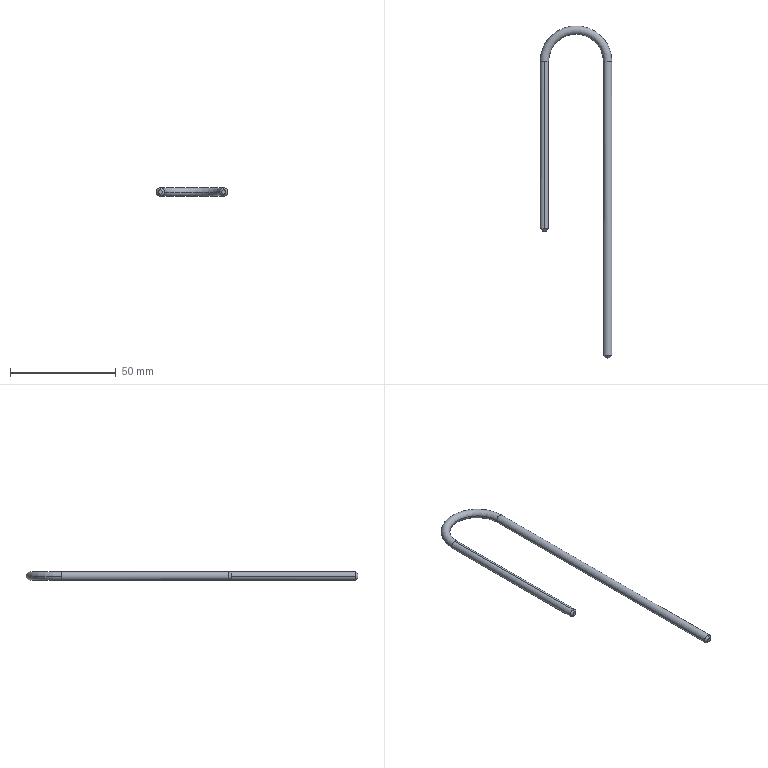Part | STEP file | MT-COMBO-119-S045 | 1 solid | 12 faces | box 34 x 157 x 4 mm | volume 3346 mm3 | cone 4 | cylinder 4 | torus 2 | plane 2 | commonest cylinder face diameters 4 x4
STEP:
#1=CARTESIAN_POINT('',(0.,80.,-2.));
#2=VERTEX_POINT('',#1);
#3=CARTESIAN_POINT('',(-2.,80.,0.));
#4=VERTEX_POINT('',#3);
#5=CARTESIAN_POINT('',(0.,80.,0.));
#6=DIRECTION('',(0.,1.,0.));
#7=DIRECTION('',(0.,0.,1.));
#8=AXIS2_PLACEMENT_3D('',#5,#6,#7);
#9=CIRCLE('',#8,2.);
#10=EDGE_CURVE('',#2,#4,#9,.T.);
#11=ORIENTED_EDGE('',*,*,#10,.T.);
#12=CARTESIAN_POINT('',(32.,80.,0.));
#13=VERTEX_POINT('',#12);
#14=CARTESIAN_POINT('',(15.,80.,0.));
#15=DIRECTION('',(0.,0.,-1.));
#16=DIRECTION('',(-1.,0.,0.));
#17=AXIS2_PLACEMENT_3D('',#14,#15,#16);
#18=CIRCLE('',#17,17.);
#19=EDGE_CURVE('',#4,#13,#18,.T.);
#20=ORIENTED_EDGE('',*,*,#19,.T.);
#21=CARTESIAN_POINT('',(28.,80.,0.));
#22=VERTEX_POINT('',#21);
#23=CARTESIAN_POINT('',(30.,80.,0.));
#24=DIRECTION('',(0.,-1.,0.));
#25=DIRECTION('',(0.,0.,1.));
#26=AXIS2_PLACEMENT_3D('',#23,#24,#25);
#27=CIRCLE('',#26,2.);
#28=EDGE_CURVE('',#22,#13,#27,.T.);
#29=ORIENTED_EDGE('',*,*,#28,.F.);
#30=CARTESIAN_POINT('',(2.,80.,0.));
#31=VERTEX_POINT('',#30);
#32=CARTESIAN_POINT('',(15.,80.,0.));
#33=DIRECTION('',(0.,0.,-1.));
#34=DIRECTION('',(-1.,0.,0.));
#35=AXIS2_PLACEMENT_3D('',#32,#33,#34);
#36=CIRCLE('',#35,13.);
#37=EDGE_CURVE('',#31,#22,#36,.T.);
#38=ORIENTED_EDGE('',*,*,#37,.F.);
#39=CARTESIAN_POINT('',(0.,80.,0.));
#40=DIRECTION('',(0.,1.,0.));
#41=DIRECTION('',(0.,0.,1.));
#42=AXIS2_PLACEMENT_3D('',#39,#40,#41);
#43=CIRCLE('',#42,2.);
#44=EDGE_CURVE('',#31,#2,#43,.T.);
#45=ORIENTED_EDGE('',*,*,#44,.T.);
#46=EDGE_LOOP('',(#11,#20,#29,#38,#45));
#47=FACE_OUTER_BOUND('',#46,.T.);
#48=CARTESIAN_POINT('',(15.,80.,0.));
#49=DIRECTION('',(0.,0.,-1.));
#50=DIRECTION('',(-1.,0.,0.));
#51=AXIS2_PLACEMENT_3D('',#48,#49,#50);
#52=TOROIDAL_SURFACE('',#51,15.,2.);
#53=ADVANCED_FACE('',(#47),#52,.T.);
#54=CARTESIAN_POINT('',(0.,0.,-1.));
#55=VERTEX_POINT('',#54);
#56=CARTESIAN_POINT('',(0.,0.,1.));
#57=VERTEX_POINT('',#56);
#58=CARTESIAN_POINT('',(0.,0.,0.));
#59=DIRECTION('',(0.,-1.,0.));
#60=DIRECTION('',(0.,0.,1.));
#61=AXIS2_PLACEMENT_3D('',#58,#59,#60);
#62=CIRCLE('',#61,1.);
#63=EDGE_CURVE('',#55,#57,#62,.T.);
#64=ORIENTED_EDGE('',*,*,#63,.F.);
#65=CARTESIAN_POINT('',(0.,1.,-2.));
#66=VERTEX_POINT('',#65);
#67=CARTESIAN_POINT('',(0.,1.,-2.));
#68=DIRECTION('',(0.,0.7071,-0.7071));
#69=VECTOR('',#68,1000.);
#70=LINE('',#67,#69);
#71=EDGE_CURVE('',#55,#66,#70,.T.);
#72=ORIENTED_EDGE('',*,*,#71,.T.);
#73=CARTESIAN_POINT('',(0.,1.,2.));
#74=VERTEX_POINT('',#73);
#75=CARTESIAN_POINT('',(0.,1.,0.));
#76=DIRECTION('',(0.,1.,0.));
#77=DIRECTION('',(0.,0.,1.));
#78=AXIS2_PLACEMENT_3D('',#75,#76,#77);
#79=CIRCLE('',#78,2.);
#80=EDGE_CURVE('',#74,#66,#79,.T.);
#81=ORIENTED_EDGE('',*,*,#80,.F.);
#82=CARTESIAN_POINT('',(0.,1.,2.));
#83=DIRECTION('',(0.,0.7071,0.7071));
#84=VECTOR('',#83,1000.);
#85=LINE('',#82,#84);
#86=EDGE_CURVE('',#57,#74,#85,.T.);
#87=ORIENTED_EDGE('',*,*,#86,.F.);
#88=EDGE_LOOP('',(#64,#72,#81,#87));
#89=FACE_OUTER_BOUND('',#88,.T.);
#90=CARTESIAN_POINT('',(0.,1.,0.));
#91=DIRECTION('',(0.,1.,0.));
#92=DIRECTION('',(0.,0.,1.));
#93=AXIS2_PLACEMENT_3D('',#90,#91,#92);
#94=CONICAL_SURFACE('',#93,2.,0.7854);
#95=ADVANCED_FACE('',(#89),#94,.T.);
#96=CARTESIAN_POINT('',(30.,-60.,-1.));
#97=VERTEX_POINT('',#96);
#98=CARTESIAN_POINT('',(30.,-60.,1.));
#99=VERTEX_POINT('',#98);
#100=CARTESIAN_POINT('',(30.,-60.,0.));
#101=DIRECTION('',(0.,-1.,0.));
#102=DIRECTION('',(1.,0.,0.));
#103=AXIS2_PLACEMENT_3D('',#100,#101,#102);
#104=CIRCLE('',#103,1.);
#105=EDGE_CURVE('',#97,#99,#104,.T.);
#106=ORIENTED_EDGE('',*,*,#105,.F.);
#107=CARTESIAN_POINT('',(30.,-59.,-2.));
#108=VERTEX_POINT('',#107);
#109=CARTESIAN_POINT('',(30.,-60.,-1.));
#110=DIRECTION('',(0.,0.7071,-0.7071));
#111=VECTOR('',#110,1000.);
#112=LINE('',#109,#111);
#113=EDGE_CURVE('',#97,#108,#112,.T.);
#114=ORIENTED_EDGE('',*,*,#113,.T.);
#115=CARTESIAN_POINT('',(32.,-59.,0.));
#116=VERTEX_POINT('',#115);
#117=CARTESIAN_POINT('',(30.,-59.,0.));
#118=DIRECTION('',(0.,1.,0.));
#119=DIRECTION('',(0.,0.,-1.));
#120=AXIS2_PLACEMENT_3D('',#117,#118,#119);
#121=CIRCLE('',#120,2.);
#122=EDGE_CURVE('',#116,#108,#121,.T.);
#123=ORIENTED_EDGE('',*,*,#122,.F.);
#124=CARTESIAN_POINT('',(30.,-59.,2.));
#125=VERTEX_POINT('',#124);
#126=CARTESIAN_POINT('',(30.,-59.,0.));
#127=DIRECTION('',(0.,1.,0.));
#128=DIRECTION('',(0.,0.,-1.));
#129=AXIS2_PLACEMENT_3D('',#126,#127,#128);
#130=CIRCLE('',#129,2.);
#131=EDGE_CURVE('',#125,#116,#130,.T.);
#132=ORIENTED_EDGE('',*,*,#131,.F.);
#133=CARTESIAN_POINT('',(30.,-60.,1.));
#134=DIRECTION('',(0.,0.7071,0.7071));
#135=VECTOR('',#134,1000.);
#136=LINE('',#133,#135);
#137=EDGE_CURVE('',#99,#125,#136,.T.);
#138=ORIENTED_EDGE('',*,*,#137,.F.);
#139=EDGE_LOOP('',(#106,#114,#123,#132,#138));
#140=FACE_OUTER_BOUND('',#139,.T.);
#141=CARTESIAN_POINT('',(30.,-60.,0.));
#142=DIRECTION('',(0.,1.,0.));
#143=DIRECTION('',(0.,0.,1.));
#144=AXIS2_PLACEMENT_3D('',#141,#142,#143);
#145=CONICAL_SURFACE('',#144,1.,0.7854);
#146=ADVANCED_FACE('',(#140),#145,.T.);
#147=CARTESIAN_POINT('',(30.,80.,0.));
#148=DIRECTION('',(0.,-1.,0.));
#149=DIRECTION('',(0.,0.,1.));
#150=AXIS2_PLACEMENT_3D('',#147,#148,#149);
#151=CIRCLE('',#150,2.);
#152=EDGE_CURVE('',#13,#22,#151,.T.);
#153=ORIENTED_EDGE('',*,*,#152,.T.);
#154=CARTESIAN_POINT('',(28.,-59.,0.));
#155=VERTEX_POINT('',#154);
#156=CARTESIAN_POINT('',(28.,80.,0.));
#157=DIRECTION('',(0.,-1.,0.));
#158=VECTOR('',#157,1000.);
#159=LINE('',#156,#158);
#160=EDGE_CURVE('',#22,#155,#159,.T.);
#161=ORIENTED_EDGE('',*,*,#160,.T.);
#162=CARTESIAN_POINT('',(30.,-59.,0.));
#163=DIRECTION('',(0.,1.,0.));
#164=DIRECTION('',(0.,0.,-1.));
#165=AXIS2_PLACEMENT_3D('',#162,#163,#164);
#166=CIRCLE('',#165,2.);
#167=EDGE_CURVE('',#155,#125,#166,.T.);
#168=ORIENTED_EDGE('',*,*,#167,.T.);
#169=ORIENTED_EDGE('',*,*,#131,.T.);
#170=CARTESIAN_POINT('',(32.,80.,0.));
#171=DIRECTION('',(0.,-1.,0.));
#172=VECTOR('',#171,1000.);
#173=LINE('',#170,#172);
#174=EDGE_CURVE('',#13,#116,#173,.T.);
#175=ORIENTED_EDGE('',*,*,#174,.F.);
#176=EDGE_LOOP('',(#153,#161,#168,#169,#175));
#177=FACE_OUTER_BOUND('',#176,.T.);
#178=CARTESIAN_POINT('',(30.,80.,0.));
#179=DIRECTION('',(0.,-1.,0.));
#180=DIRECTION('',(1.,0.,0.));
#181=AXIS2_PLACEMENT_3D('',#178,#179,#180);
#182=CYLINDRICAL_SURFACE('',#181,2.);
#183=ADVANCED_FACE('',(#177),#182,.T.);
#184=ORIENTED_EDGE('',*,*,#80,.T.);
#185=CARTESIAN_POINT('',(0.,0.,-2.));
#186=DIRECTION('',(0.,1.,0.));
#187=VECTOR('',#186,1000.);
#188=LINE('',#185,#187);
#189=EDGE_CURVE('',#66,#2,#188,.T.);
#190=ORIENTED_EDGE('',*,*,#189,.T.);
#191=ORIENTED_EDGE('',*,*,#44,.F.);
#192=CARTESIAN_POINT('',(0.,80.,2.));
#193=VERTEX_POINT('',#192);
#194=CARTESIAN_POINT('',(0.,80.,0.));
#195=DIRECTION('',(0.,1.,0.));
#196=DIRECTION('',(0.,0.,1.));
#197=AXIS2_PLACEMENT_3D('',#194,#195,#196);
#198=CIRCLE('',#197,2.);
#199=EDGE_CURVE('',#193,#31,#198,.T.);
#200=ORIENTED_EDGE('',*,*,#199,.F.);
#201=CARTESIAN_POINT('',(0.,0.,2.));
#202=DIRECTION('',(0.,1.,0.));
#203=VECTOR('',#202,1000.);
#204=LINE('',#201,#203);
#205=EDGE_CURVE('',#74,#193,#204,.T.);
#206=ORIENTED_EDGE('',*,*,#205,.F.);
#207=EDGE_LOOP('',(#184,#190,#191,#200,#206));
#208=FACE_OUTER_BOUND('',#207,.T.);
#209=CARTESIAN_POINT('',(0.,0.,0.));
#210=DIRECTION('',(0.,1.,0.));
#211=DIRECTION('',(0.,0.,1.));
#212=AXIS2_PLACEMENT_3D('',#209,#210,#211);
#213=CYLINDRICAL_SURFACE('',#212,2.);
#214=ADVANCED_FACE('',(#208),#213,.T.);
#215=ORIENTED_EDGE('',*,*,#160,.F.);
#216=ORIENTED_EDGE('',*,*,#28,.T.);
#217=ORIENTED_EDGE('',*,*,#174,.T.);
#218=ORIENTED_EDGE('',*,*,#122,.T.);
#219=CARTESIAN_POINT('',(30.,-59.,0.));
#220=DIRECTION('',(0.,1.,0.));
#221=DIRECTION('',(0.,0.,-1.));
#222=AXIS2_PLACEMENT_3D('',#219,#220,#221);
#223=CIRCLE('',#222,2.);
#224=EDGE_CURVE('',#108,#155,#223,.T.);
#225=ORIENTED_EDGE('',*,*,#224,.T.);
#226=EDGE_LOOP('',(#215,#216,#217,#218,#225));
#227=FACE_OUTER_BOUND('',#226,.T.);
#228=CARTESIAN_POINT('',(30.,80.,0.));
#229=DIRECTION('',(0.,-1.,0.));
#230=DIRECTION('',(1.,0.,0.));
#231=AXIS2_PLACEMENT_3D('',#228,#229,#230);
#232=CYLINDRICAL_SURFACE('',#231,2.);
#233=ADVANCED_FACE('',(#227),#232,.T.);
#234=ORIENTED_EDGE('',*,*,#19,.F.);
#235=CARTESIAN_POINT('',(0.,80.,0.));
#236=DIRECTION('',(0.,1.,0.));
#237=DIRECTION('',(0.,0.,1.));
#238=AXIS2_PLACEMENT_3D('',#235,#236,#237);
#239=CIRCLE('',#238,2.);
#240=EDGE_CURVE('',#4,#193,#239,.T.);
#241=ORIENTED_EDGE('',*,*,#240,.T.);
#242=ORIENTED_EDGE('',*,*,#199,.T.);
#243=ORIENTED_EDGE('',*,*,#37,.T.);
#244=ORIENTED_EDGE('',*,*,#152,.F.);
#245=EDGE_LOOP('',(#234,#241,#242,#243,#244));
#246=FACE_OUTER_BOUND('',#245,.T.);
#247=CARTESIAN_POINT('',(15.,80.,0.));
#248=DIRECTION('',(0.,0.,-1.));
#249=DIRECTION('',(-1.,0.,0.));
#250=AXIS2_PLACEMENT_3D('',#247,#248,#249);
#251=TOROIDAL_SURFACE('',#250,15.,2.);
#252=ADVANCED_FACE('',(#246),#251,.T.);
#253=ORIENTED_EDGE('',*,*,#189,.F.);
#254=CARTESIAN_POINT('',(0.,1.,0.));
#255=DIRECTION('',(0.,1.,0.));
#256=DIRECTION('',(0.,0.,1.));
#257=AXIS2_PLACEMENT_3D('',#254,#255,#256);
#258=CIRCLE('',#257,2.);
#259=EDGE_CURVE('',#66,#74,#258,.T.);
#260=ORIENTED_EDGE('',*,*,#259,.T.);
#261=ORIENTED_EDGE('',*,*,#205,.T.);
#262=ORIENTED_EDGE('',*,*,#240,.F.);
#263=ORIENTED_EDGE('',*,*,#10,.F.);
#264=EDGE_LOOP('',(#253,#260,#261,#262,#263));
#265=FACE_OUTER_BOUND('',#264,.T.);
#266=CARTESIAN_POINT('',(0.,0.,0.));
#267=DIRECTION('',(0.,1.,0.));
#268=DIRECTION('',(0.,0.,1.));
#269=AXIS2_PLACEMENT_3D('',#266,#267,#268);
#270=CYLINDRICAL_SURFACE('',#269,2.);
#271=ADVANCED_FACE('',(#265),#270,.T.);
#272=CARTESIAN_POINT('',(30.,-60.,0.));
#273=DIRECTION('',(0.,-1.,0.));
#274=DIRECTION('',(1.,0.,0.));
#275=AXIS2_PLACEMENT_3D('',#272,#273,#274);
#276=CIRCLE('',#275,1.);
#277=EDGE_CURVE('',#99,#97,#276,.T.);
#278=ORIENTED_EDGE('',*,*,#277,.T.);
#279=ORIENTED_EDGE('',*,*,#105,.T.);
#280=EDGE_LOOP('',(#278,#279));
#281=FACE_OUTER_BOUND('',#280,.T.);
#282=CARTESIAN_POINT('',(30.,-60.,0.));
#283=DIRECTION('',(0.,-1.,0.));
#284=DIRECTION('',(0.,0.,1.));
#285=AXIS2_PLACEMENT_3D('',#282,#283,#284);
#286=PLANE('',#285);
#287=ADVANCED_FACE('',(#281),#286,.T.);
#288=CARTESIAN_POINT('',(0.,0.,0.));
#289=DIRECTION('',(0.,-1.,0.));
#290=DIRECTION('',(0.,0.,1.));
#291=AXIS2_PLACEMENT_3D('',#288,#289,#290);
#292=CIRCLE('',#291,1.);
#293=EDGE_CURVE('',#57,#55,#292,.T.);
#294=ORIENTED_EDGE('',*,*,#293,.T.);
#295=ORIENTED_EDGE('',*,*,#63,.T.);
#296=EDGE_LOOP('',(#294,#295));
#297=FACE_OUTER_BOUND('',#296,.T.);
#298=CARTESIAN_POINT('',(0.,0.,0.));
#299=DIRECTION('',(0.,1.,0.));
#300=DIRECTION('',(0.,0.,1.));
#301=AXIS2_PLACEMENT_3D('',#298,#299,#300);
#302=PLANE('',#301);
#303=ADVANCED_FACE('',(#297),#302,.F.);
#304=ORIENTED_EDGE('',*,*,#113,.F.);
#305=ORIENTED_EDGE('',*,*,#277,.F.);
#306=ORIENTED_EDGE('',*,*,#137,.T.);
#307=ORIENTED_EDGE('',*,*,#167,.F.);
#308=ORIENTED_EDGE('',*,*,#224,.F.);
#309=EDGE_LOOP('',(#304,#305,#306,#307,#308));
#310=FACE_OUTER_BOUND('',#309,.T.);
#311=CARTESIAN_POINT('',(30.,-60.,0.));
#312=DIRECTION('',(0.,1.,0.));
#313=DIRECTION('',(0.,0.,1.));
#314=AXIS2_PLACEMENT_3D('',#311,#312,#313);
#315=CONICAL_SURFACE('',#314,1.,0.7854);
#316=ADVANCED_FACE('',(#310),#315,.T.);
#317=ORIENTED_EDGE('',*,*,#71,.F.);
#318=ORIENTED_EDGE('',*,*,#293,.F.);
#319=ORIENTED_EDGE('',*,*,#86,.T.);
#320=ORIENTED_EDGE('',*,*,#259,.F.);
#321=EDGE_LOOP('',(#317,#318,#319,#320));
#322=FACE_OUTER_BOUND('',#321,.T.);
#323=CARTESIAN_POINT('',(0.,1.,0.));
#324=DIRECTION('',(0.,1.,0.));
#325=DIRECTION('',(0.,0.,1.));
#326=AXIS2_PLACEMENT_3D('',#323,#324,#325);
#327=CONICAL_SURFACE('',#326,2.,0.7854);
#328=ADVANCED_FACE('',(#322),#327,.T.);
#329=CLOSED_SHELL('',(#53,#95,#146,#183,#214,#233,#252,#271,#287,#303,#316,#328));
#330=MANIFOLD_SOLID_BREP('',#329);
#331=CARTESIAN_POINT('',(0.,0.,0.));
#332=DIRECTION('',(0.,0.,1.));
#333=DIRECTION('',(1.,0.,0.));
#334=AXIS2_PLACEMENT_3D('',#331,#332,#333);
#335=(LENGTH_UNIT()NAMED_UNIT(*)SI_UNIT(.MILLI.,.METRE.));
#336=UNCERTAINTY_MEASURE_WITH_UNIT(LENGTH_MEASURE(0.00001),#335,'','');
#337=(NAMED_UNIT(*)PLANE_ANGLE_UNIT()SI_UNIT($,.RADIAN.));
#338=(NAMED_UNIT(*)SI_UNIT($,.STERADIAN.)SOLID_ANGLE_UNIT());
#339=(GEOMETRIC_REPRESENTATION_CONTEXT(3)GLOBAL_UNCERTAINTY_ASSIGNED_CONTEXT((#336))GLOBAL_UNIT_ASSIGNED_CONTEXT((#335,#337,#338))REPRESENTATION_CONTEXT('',''));
#340=ADVANCED_BREP_SHAPE_REPRESENTATION('',(#330,#334),#339);